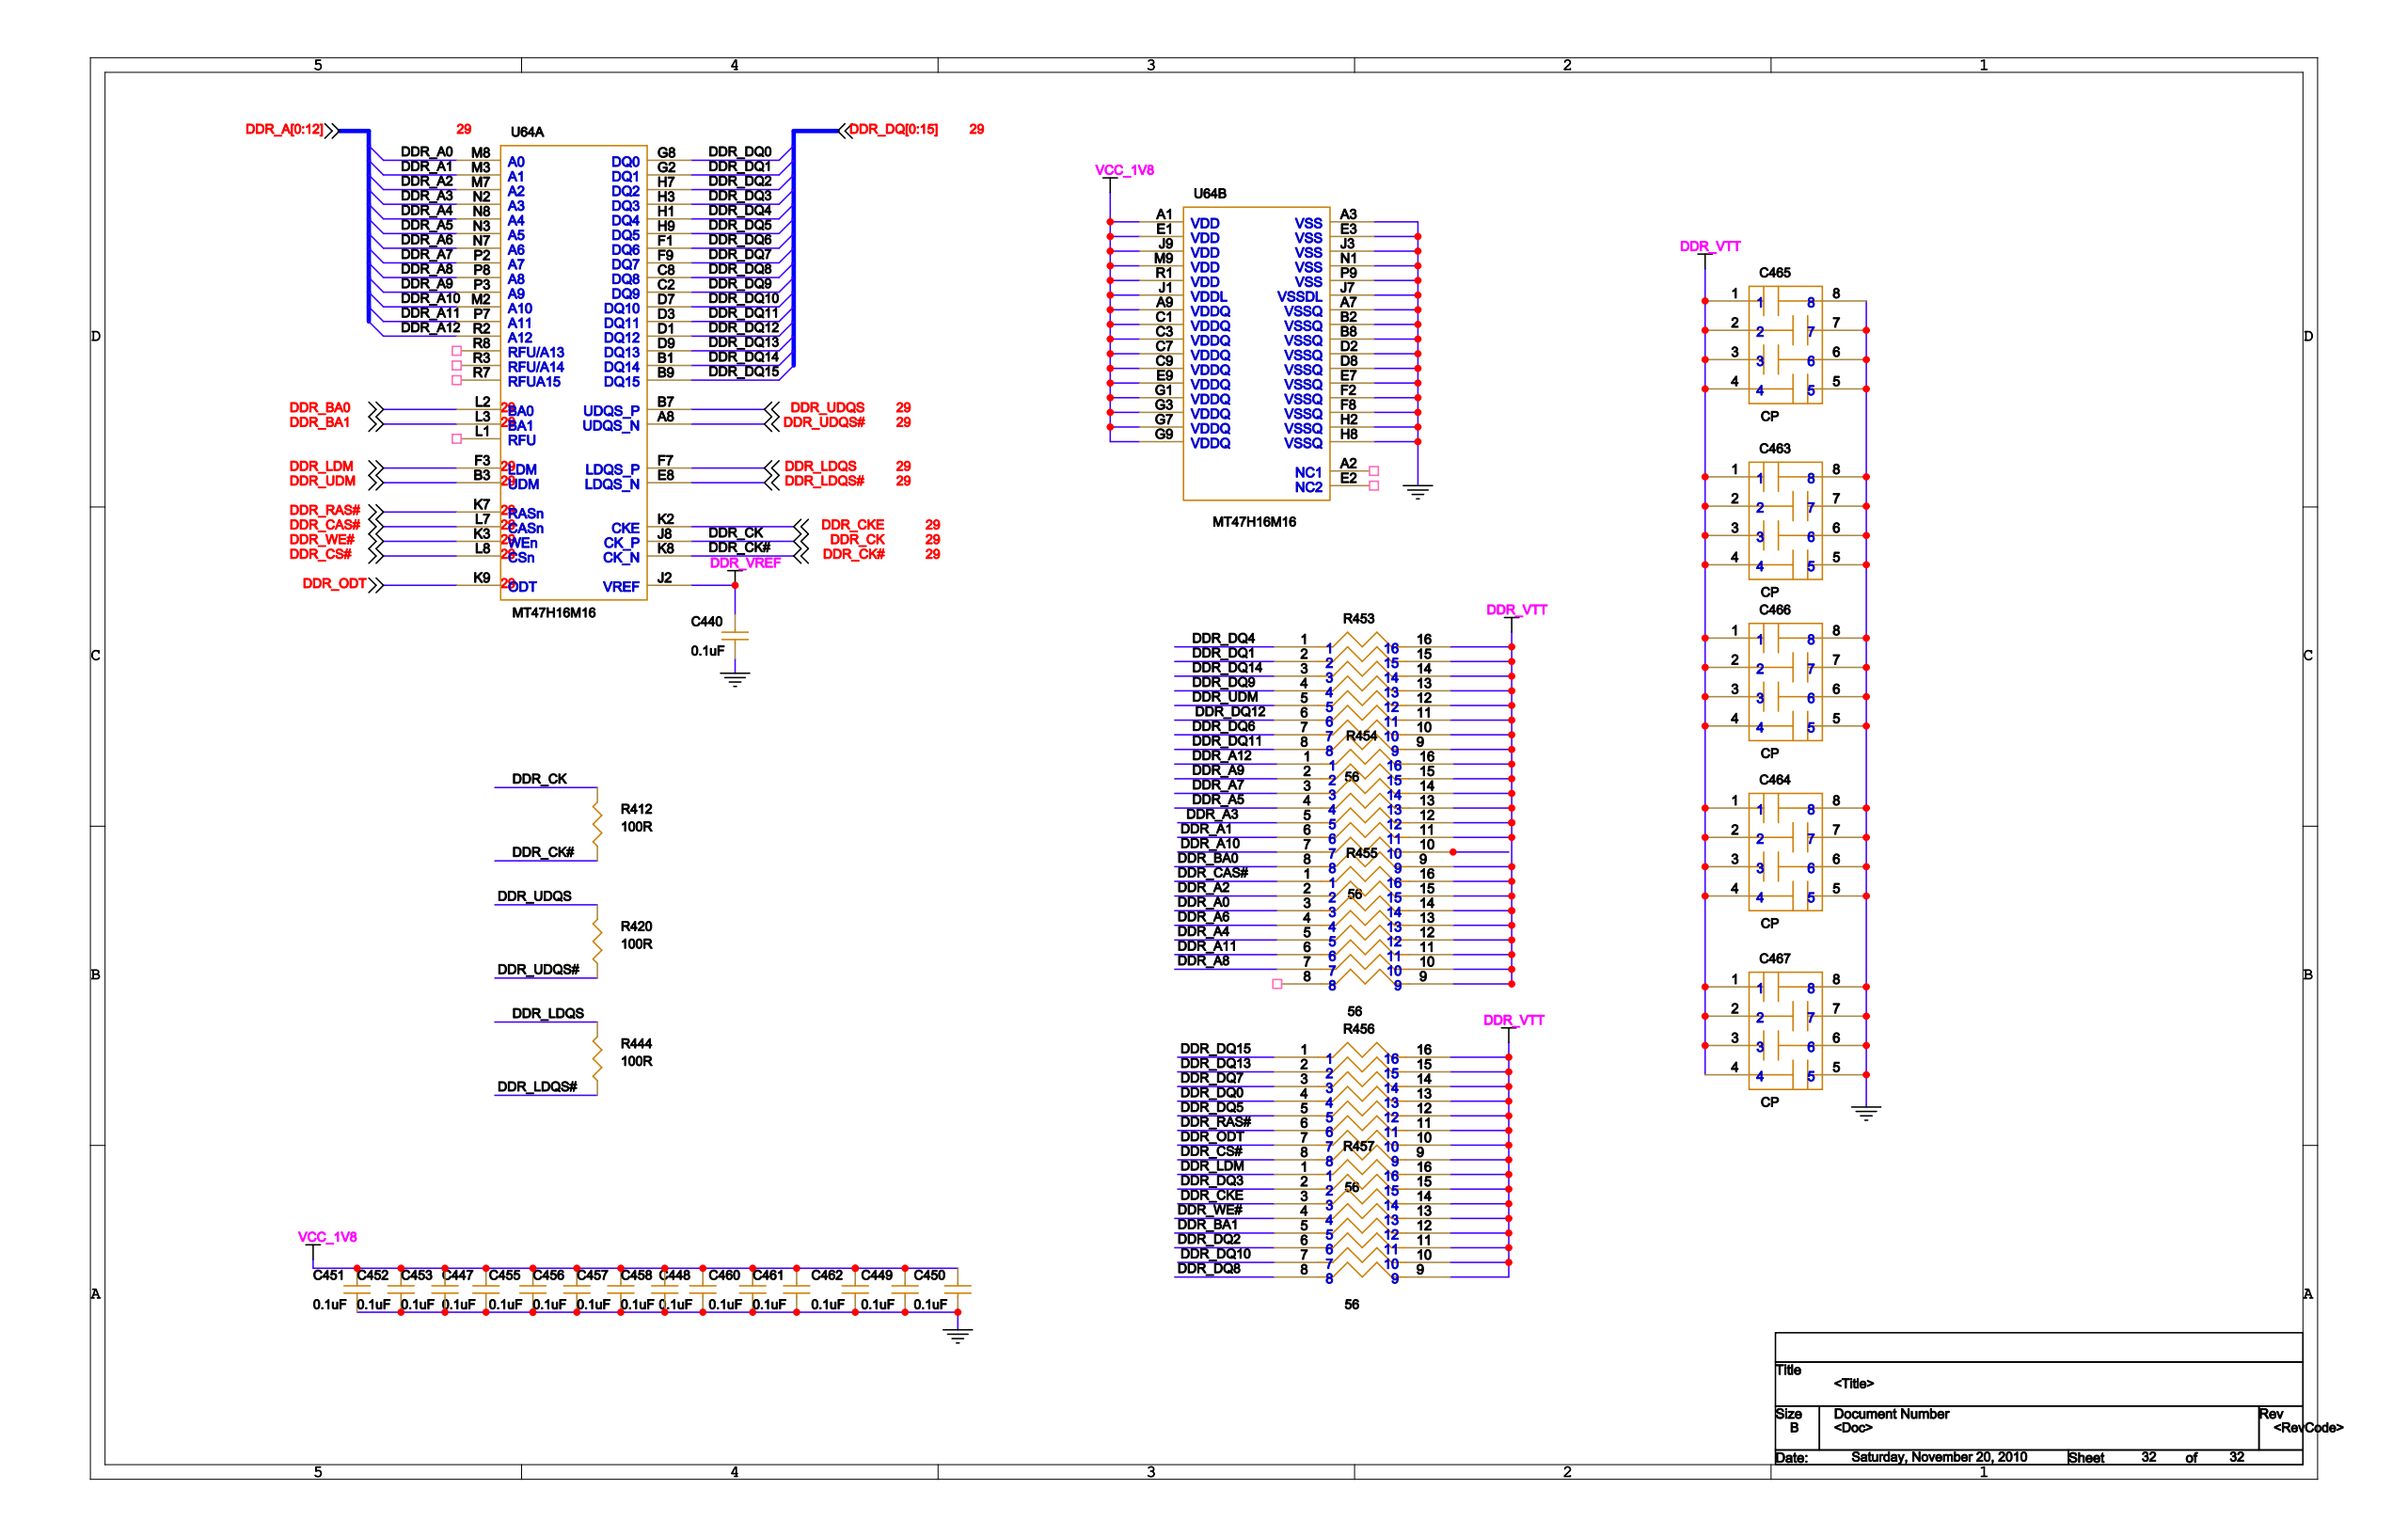Circuit board | Cadence Allegro | 1001 parts | 1318 nets | one sheet of the schematic
Parts on this sheet (reference | value | footprint):
C440 | 0.1uF | C0402
C447 | 0.1uF | C0402
C448 | 0.1uF | C0402
C449 | 0.1uF | C0402
C450 | 0.1uF | C0402
C451 | 0.1uF | C0402
C452 | 0.1uF | C0402
C453 | 0.1uF | C0402
C455 | 0.1uF | C0402
C456 | 0.1uF | C0402
C457 | 0.1uF | C0402
C458 | 0.1uF | C0402
C460 | 0.1uF | C0402
C461 | 0.1uF | C0402
C462 | 0.1uF | C0402
C463 | CP | CA-AVE-0603-8
C464 | CP | CA-AVE-0603-8
C465 | CP | CA-AVE-0603-8
C466 | CP | CA-AVE-0603-8
C467 | CP | CA-AVE-0603-8
R412 | 100R | C0402
R420 | 100R | C0402
R444 | 100R | C0402
R453 | 56 | RA-VEX-0603-16
R454 | 56 | RA-VEX-0603-16
R455 | 56 | RA-VEX-0603-16
R456 | 56 | RA-VEX-0603-16
R457 | 56 | RA-VEX-0603-16
U64 | MT47H16M16 | FBGA-84
Nets of these parts (net: part-pin ...):
DDR_DQ14: R453-3 U64-B1
DDR_DQ12: R453-6 U64-D1
DDR_DQ6: R453-7 U64-F1
DDR_DQ9: R453-4 U64-C2
DDR_DQ4: R453-1 U64-H1
DDR_DQ3: R457-2 U64-H3
DDR_DQ1: R453-2 U64-G2
DDR_LDM: R457-1 U64-F3
DDR_DQ11: R453-8 U64-D3
DDR_DQ2: R457-6 U64-H7
DDR_UDM: R453-5 U64-B3
DDR_DQ5: R456-5 U64-H9
DDR_CK#: R412-1 U64-K8
DDR_DQ13: R456-2 U64-D9
DDR_DQ10: R457-7 U64-D7
DDR_UDQS#: R420-1 U64-A8
DDR_CK: R412-2 U64-J8
DDR_DQ15: R456-1 U64-B9
DDR_DQ8: R457-8 U64-C8
DDR_DQ7: R456-3 U64-F9
DDR_DQ0: R456-4 U64-G8
DDR_UDQS: R420-2 U64-B7
DDR_CKE: R457-3 U64-K2
DDR_A10: R454-7 U64-M2
DDR_A9: R454-2 U64-P3
DDR_BA0: R454-8 U64-L2
DDR_A12: R454-1 U64-R2
DDR_A3: R454-5 U64-N2
DDR_A7: R454-3 U64-P2
DDR_WE#: R457-4 U64-K3
DDR_A5: R454-4 U64-N3
DDR_BA1: R457-5 U64-L3
DDR_A11: R455-6 U64-P7
DDR_A1: R454-6 U64-M3
DDR_A8: R455-7 U64-P8
DDR_ODT: R456-7 U64-K9
DDR_CAS#: R455-1 U64-L7
DDR_A6: R455-4 U64-N7
DDR_RAS#: R456-6 U64-K7
DDR_A2: R455-2 U64-M7
DDR_A4: R455-5 U64-N8
DDR_LDQS: R444-2 U64-F7
DDR_LDQS#: R444-1 U64-E8
DDR_CS#: R456-8 U64-L8
DDR_A0: R455-3 U64-M8
GND: C440-2 C447-2 C448-2 C449-2 C450-2 C451-2 C452-2 C453-2 C455-2 C456-2 C457-2 C458-2 C460-2 C461-2 C462-2 C463-5 C463-6 C463-7 C463-8 C464-5 C464-6 C464-7 C464-8 C465-5 C465-6 C465-7 C465-8 C466-5 C466-6 C466-7 C466-8 C467-5 C467-6 C467-7 C467-8 U64-A3 U64-A7 U64-B2 U64-B8 U64-D2 U64-D8 U64-E3 U64-E7 U64-F2 U64-F8 U64-H2 U64-H8 U64-J3 U64-J7 U64-N1 U64-P9
VCC_1V8: C447-1 C448-1 C449-1 C450-1 C451-1 C452-1 C453-1 C455-1 C456-1 C457-1 C458-1 C460-1 C461-1 C462-1 U64-A1 U64-A9 U64-C1 U64-C3 U64-C7 U64-C9 U64-E1 U64-E9 U64-G1 U64-G3 U64-G7 U64-G9 U64-J1 U64-J9 U64-M9 U64-R1
DDR_VREF: C440-1 U64-J2
DDR_VTT: C463-1 C463-2 C463-3 C463-4 C464-1 C464-2 C464-3 C464-4 C465-1 C465-2 C465-3 C465-4 C466-1 C466-2 C466-3 C466-4 C467-1 C467-2 C467-3 C467-4 R453-9 R453-10 R453-11 R453-12 R453-13 R453-14 R453-15 R453-16 R454-9 R454-11 R454-12 R454-13 R454-14 R454-15 R454-16 R455-9 R455-10 R455-11 R455-12 R455-13 R455-14 R455-15 R455-16 R456-9 R456-10 R456-11 R456-12 R456-13 R456-14 R456-15 R456-16 R457-9 R457-10 R457-11 R457-12 R457-13 R457-14 R457-15 R457-16
N18700915: R454-10